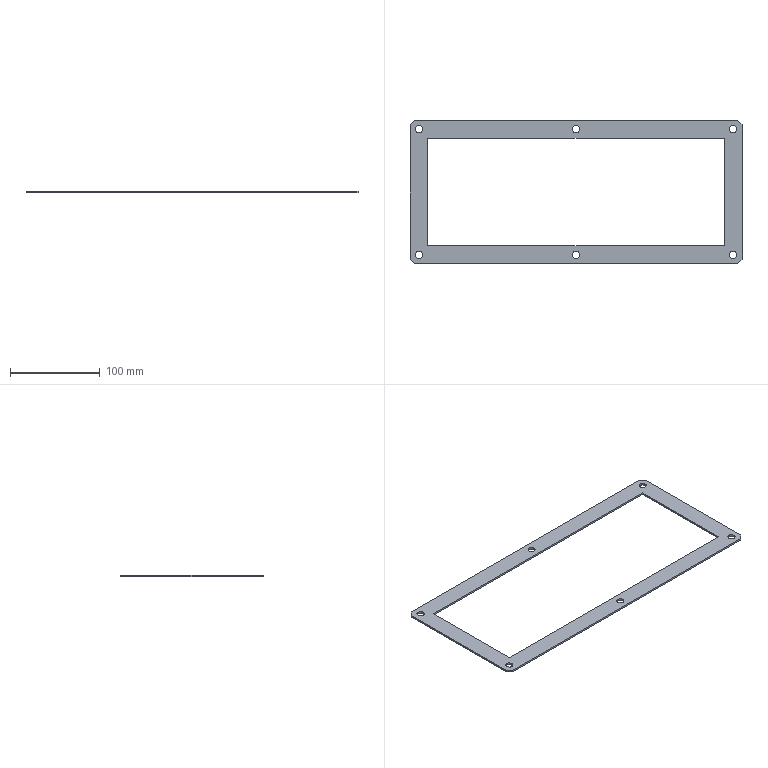Part | STEP file | SYL_0392D6J1SYL0380DJ10-1368501 | 1 solid | 26 faces | box 370 x 160 x 2 mm | volume 38497 mm3 | plane 14 | cylinder 12 | commonest cylinder face diameters 8 x12
STEP:
#1=CARTESIAN_POINT('',(-171.,70.,-2.));
#2=VERTEX_POINT('',#1);
#3=CARTESIAN_POINT('',(-179.,70.,-2.));
#4=VERTEX_POINT('',#3);
#5=CARTESIAN_POINT('',(-175.,70.,-2.));
#6=DIRECTION('',(0.,0.,1.));
#7=DIRECTION('',(1.,0.,0.));
#8=AXIS2_PLACEMENT_3D('',#5,#6,#7);
#9=CIRCLE('',#8,4.);
#10=EDGE_CURVE('',#2,#4,#9,.T.);
#11=ORIENTED_EDGE('',*,*,#10,.F.);
#12=CARTESIAN_POINT('',(-171.,70.,0.));
#13=VERTEX_POINT('',#12);
#14=CARTESIAN_POINT('',(-171.,70.,0.));
#15=DIRECTION('',(0.,0.,-1.));
#16=VECTOR('',#15,1000.);
#17=LINE('',#14,#16);
#18=EDGE_CURVE('',#13,#2,#17,.T.);
#19=ORIENTED_EDGE('',*,*,#18,.F.);
#20=CARTESIAN_POINT('',(-179.,70.,0.));
#21=VERTEX_POINT('',#20);
#22=CARTESIAN_POINT('',(-175.,70.,0.));
#23=DIRECTION('',(0.,0.,-1.));
#24=DIRECTION('',(-1.,0.,0.));
#25=AXIS2_PLACEMENT_3D('',#22,#23,#24);
#26=CIRCLE('',#25,4.);
#27=EDGE_CURVE('',#21,#13,#26,.T.);
#28=ORIENTED_EDGE('',*,*,#27,.F.);
#29=CARTESIAN_POINT('',(-179.,70.,0.));
#30=DIRECTION('',(0.,0.,-1.));
#31=VECTOR('',#30,1000.);
#32=LINE('',#29,#31);
#33=EDGE_CURVE('',#21,#4,#32,.T.);
#34=ORIENTED_EDGE('',*,*,#33,.T.);
#35=EDGE_LOOP('',(#11,#19,#28,#34));
#36=FACE_OUTER_BOUND('',#35,.T.);
#37=CARTESIAN_POINT('',(-175.,70.,-1.));
#38=DIRECTION('',(0.,0.,1.));
#39=DIRECTION('',(1.,0.,0.));
#40=AXIS2_PLACEMENT_3D('',#37,#38,#39);
#41=CYLINDRICAL_SURFACE('',#40,4.);
#42=ADVANCED_FACE('',(#36),#41,.F.);
#43=ORIENTED_EDGE('',*,*,#33,.F.);
#44=CARTESIAN_POINT('',(-175.,70.,0.));
#45=DIRECTION('',(0.,0.,-1.));
#46=DIRECTION('',(1.,0.,0.));
#47=AXIS2_PLACEMENT_3D('',#44,#45,#46);
#48=CIRCLE('',#47,4.);
#49=EDGE_CURVE('',#13,#21,#48,.T.);
#50=ORIENTED_EDGE('',*,*,#49,.F.);
#51=ORIENTED_EDGE('',*,*,#18,.T.);
#52=CARTESIAN_POINT('',(-175.,70.,-2.));
#53=DIRECTION('',(0.,0.,1.));
#54=DIRECTION('',(-1.,0.,0.));
#55=AXIS2_PLACEMENT_3D('',#52,#53,#54);
#56=CIRCLE('',#55,4.);
#57=EDGE_CURVE('',#4,#2,#56,.T.);
#58=ORIENTED_EDGE('',*,*,#57,.F.);
#59=EDGE_LOOP('',(#43,#50,#51,#58));
#60=FACE_OUTER_BOUND('',#59,.T.);
#61=CARTESIAN_POINT('',(-175.,70.,-1.));
#62=DIRECTION('',(0.,0.,1.));
#63=DIRECTION('',(1.,0.,0.));
#64=AXIS2_PLACEMENT_3D('',#61,#62,#63);
#65=CYLINDRICAL_SURFACE('',#64,4.);
#66=ADVANCED_FACE('',(#60),#65,.F.);
#67=CARTESIAN_POINT('',(165.,-60.,0.));
#68=VERTEX_POINT('',#67);
#69=CARTESIAN_POINT('',(-165.,-60.,0.));
#70=VERTEX_POINT('',#69);
#71=CARTESIAN_POINT('',(165.,-60.,0.));
#72=DIRECTION('',(-1.,0.,0.));
#73=VECTOR('',#72,1000.);
#74=LINE('',#71,#73);
#75=EDGE_CURVE('',#68,#70,#74,.T.);
#76=ORIENTED_EDGE('',*,*,#75,.F.);
#77=CARTESIAN_POINT('',(165.,-60.,-2.));
#78=VERTEX_POINT('',#77);
#79=CARTESIAN_POINT('',(165.,-60.,-2.));
#80=DIRECTION('',(0.,0.,1.));
#81=VECTOR('',#80,1000.);
#82=LINE('',#79,#81);
#83=EDGE_CURVE('',#78,#68,#82,.T.);
#84=ORIENTED_EDGE('',*,*,#83,.F.);
#85=CARTESIAN_POINT('',(-165.,-60.,-2.));
#86=VERTEX_POINT('',#85);
#87=CARTESIAN_POINT('',(-165.,-60.,-2.));
#88=DIRECTION('',(1.,0.,0.));
#89=VECTOR('',#88,1000.);
#90=LINE('',#87,#89);
#91=EDGE_CURVE('',#86,#78,#90,.T.);
#92=ORIENTED_EDGE('',*,*,#91,.F.);
#93=CARTESIAN_POINT('',(-165.,-60.,-2.));
#94=DIRECTION('',(0.,0.,1.));
#95=VECTOR('',#94,1000.);
#96=LINE('',#93,#95);
#97=EDGE_CURVE('',#86,#70,#96,.T.);
#98=ORIENTED_EDGE('',*,*,#97,.T.);
#99=EDGE_LOOP('',(#76,#84,#92,#98));
#100=FACE_OUTER_BOUND('',#99,.T.);
#101=CARTESIAN_POINT('',(0.,-60.,-1.));
#102=DIRECTION('',(0.,1.,0.));
#103=DIRECTION('',(1.,0.,0.));
#104=AXIS2_PLACEMENT_3D('',#101,#102,#103);
#105=PLANE('',#104);
#106=ADVANCED_FACE('',(#100),#105,.T.);
#107=CARTESIAN_POINT('',(165.,60.,0.));
#108=VERTEX_POINT('',#107);
#109=CARTESIAN_POINT('',(165.,60.,0.));
#110=DIRECTION('',(0.,-1.,0.));
#111=VECTOR('',#110,1000.);
#112=LINE('',#109,#111);
#113=EDGE_CURVE('',#108,#68,#112,.T.);
#114=ORIENTED_EDGE('',*,*,#113,.F.);
#115=CARTESIAN_POINT('',(165.,60.,-2.));
#116=VERTEX_POINT('',#115);
#117=CARTESIAN_POINT('',(165.,60.,-2.));
#118=DIRECTION('',(0.,0.,1.));
#119=VECTOR('',#118,1000.);
#120=LINE('',#117,#119);
#121=EDGE_CURVE('',#116,#108,#120,.T.);
#122=ORIENTED_EDGE('',*,*,#121,.F.);
#123=CARTESIAN_POINT('',(165.,-60.,-2.));
#124=DIRECTION('',(0.,1.,0.));
#125=VECTOR('',#124,1000.);
#126=LINE('',#123,#125);
#127=EDGE_CURVE('',#78,#116,#126,.T.);
#128=ORIENTED_EDGE('',*,*,#127,.F.);
#129=ORIENTED_EDGE('',*,*,#83,.T.);
#130=EDGE_LOOP('',(#114,#122,#128,#129));
#131=FACE_OUTER_BOUND('',#130,.T.);
#132=CARTESIAN_POINT('',(165.,0.,-1.));
#133=DIRECTION('',(-1.,0.,0.));
#134=DIRECTION('',(0.,0.,1.));
#135=AXIS2_PLACEMENT_3D('',#132,#133,#134);
#136=PLANE('',#135);
#137=ADVANCED_FACE('',(#131),#136,.T.);
#138=CARTESIAN_POINT('',(-165.,60.,0.));
#139=VERTEX_POINT('',#138);
#140=CARTESIAN_POINT('',(-165.,60.,0.));
#141=DIRECTION('',(1.,0.,0.));
#142=VECTOR('',#141,1000.);
#143=LINE('',#140,#142);
#144=EDGE_CURVE('',#139,#108,#143,.T.);
#145=ORIENTED_EDGE('',*,*,#144,.F.);
#146=CARTESIAN_POINT('',(-165.,60.,-2.));
#147=VERTEX_POINT('',#146);
#148=CARTESIAN_POINT('',(-165.,60.,0.));
#149=DIRECTION('',(0.,0.,-1.));
#150=VECTOR('',#149,1000.);
#151=LINE('',#148,#150);
#152=EDGE_CURVE('',#139,#147,#151,.T.);
#153=ORIENTED_EDGE('',*,*,#152,.T.);
#154=CARTESIAN_POINT('',(165.,60.,-2.));
#155=DIRECTION('',(-1.,0.,0.));
#156=VECTOR('',#155,1000.);
#157=LINE('',#154,#156);
#158=EDGE_CURVE('',#116,#147,#157,.T.);
#159=ORIENTED_EDGE('',*,*,#158,.F.);
#160=ORIENTED_EDGE('',*,*,#121,.T.);
#161=EDGE_LOOP('',(#145,#153,#159,#160));
#162=FACE_OUTER_BOUND('',#161,.T.);
#163=CARTESIAN_POINT('',(0.,60.,-1.));
#164=DIRECTION('',(0.,-1.,0.));
#165=DIRECTION('',(0.,0.,-1.));
#166=AXIS2_PLACEMENT_3D('',#163,#164,#165);
#167=PLANE('',#166);
#168=ADVANCED_FACE('',(#162),#167,.T.);
#169=CARTESIAN_POINT('',(-165.,-60.,0.));
#170=DIRECTION('',(0.,1.,0.));
#171=VECTOR('',#170,1000.);
#172=LINE('',#169,#171);
#173=EDGE_CURVE('',#70,#139,#172,.T.);
#174=ORIENTED_EDGE('',*,*,#173,.F.);
#175=ORIENTED_EDGE('',*,*,#97,.F.);
#176=CARTESIAN_POINT('',(-165.,60.,-2.));
#177=DIRECTION('',(0.,-1.,0.));
#178=VECTOR('',#177,1000.);
#179=LINE('',#176,#178);
#180=EDGE_CURVE('',#147,#86,#179,.T.);
#181=ORIENTED_EDGE('',*,*,#180,.F.);
#182=ORIENTED_EDGE('',*,*,#152,.F.);
#183=EDGE_LOOP('',(#174,#175,#181,#182));
#184=FACE_OUTER_BOUND('',#183,.T.);
#185=CARTESIAN_POINT('',(-165.,0.,-1.));
#186=DIRECTION('',(1.,0.,0.));
#187=DIRECTION('',(0.,1.,0.));
#188=AXIS2_PLACEMENT_3D('',#185,#186,#187);
#189=PLANE('',#188);
#190=ADVANCED_FACE('',(#184),#189,.T.);
#191=CARTESIAN_POINT('',(179.,-70.,-2.));
#192=VERTEX_POINT('',#191);
#193=CARTESIAN_POINT('',(171.,-70.,-2.));
#194=VERTEX_POINT('',#193);
#195=CARTESIAN_POINT('',(175.,-70.,-2.));
#196=DIRECTION('',(0.,0.,1.));
#197=DIRECTION('',(1.,0.,0.));
#198=AXIS2_PLACEMENT_3D('',#195,#196,#197);
#199=CIRCLE('',#198,4.);
#200=EDGE_CURVE('',#192,#194,#199,.T.);
#201=ORIENTED_EDGE('',*,*,#200,.F.);
#202=CARTESIAN_POINT('',(179.,-70.,0.));
#203=VERTEX_POINT('',#202);
#204=CARTESIAN_POINT('',(179.,-70.,0.));
#205=DIRECTION('',(0.,0.,-1.));
#206=VECTOR('',#205,1000.);
#207=LINE('',#204,#206);
#208=EDGE_CURVE('',#203,#192,#207,.T.);
#209=ORIENTED_EDGE('',*,*,#208,.F.);
#210=CARTESIAN_POINT('',(171.,-70.,0.));
#211=VERTEX_POINT('',#210);
#212=CARTESIAN_POINT('',(175.,-70.,0.));
#213=DIRECTION('',(0.,0.,-1.));
#214=DIRECTION('',(-1.,0.,0.));
#215=AXIS2_PLACEMENT_3D('',#212,#213,#214);
#216=CIRCLE('',#215,4.);
#217=EDGE_CURVE('',#211,#203,#216,.T.);
#218=ORIENTED_EDGE('',*,*,#217,.F.);
#219=CARTESIAN_POINT('',(171.,-70.,0.));
#220=DIRECTION('',(0.,0.,-1.));
#221=VECTOR('',#220,1000.);
#222=LINE('',#219,#221);
#223=EDGE_CURVE('',#211,#194,#222,.T.);
#224=ORIENTED_EDGE('',*,*,#223,.T.);
#225=EDGE_LOOP('',(#201,#209,#218,#224));
#226=FACE_OUTER_BOUND('',#225,.T.);
#227=CARTESIAN_POINT('',(175.,-70.,-1.));
#228=DIRECTION('',(0.,0.,1.));
#229=DIRECTION('',(1.,0.,0.));
#230=AXIS2_PLACEMENT_3D('',#227,#228,#229);
#231=CYLINDRICAL_SURFACE('',#230,4.);
#232=ADVANCED_FACE('',(#226),#231,.F.);
#233=CARTESIAN_POINT('',(4.,-70.,-2.));
#234=VERTEX_POINT('',#233);
#235=CARTESIAN_POINT('',(-4.,-70.,-2.));
#236=VERTEX_POINT('',#235);
#237=CARTESIAN_POINT('',(0.,-70.,-2.));
#238=DIRECTION('',(0.,0.,1.));
#239=DIRECTION('',(1.,0.,0.));
#240=AXIS2_PLACEMENT_3D('',#237,#238,#239);
#241=CIRCLE('',#240,4.);
#242=EDGE_CURVE('',#234,#236,#241,.T.);
#243=ORIENTED_EDGE('',*,*,#242,.F.);
#244=CARTESIAN_POINT('',(4.,-70.,0.));
#245=VERTEX_POINT('',#244);
#246=CARTESIAN_POINT('',(4.,-70.,0.));
#247=DIRECTION('',(0.,0.,-1.));
#248=VECTOR('',#247,1000.);
#249=LINE('',#246,#248);
#250=EDGE_CURVE('',#245,#234,#249,.T.);
#251=ORIENTED_EDGE('',*,*,#250,.F.);
#252=CARTESIAN_POINT('',(-4.,-70.,0.));
#253=VERTEX_POINT('',#252);
#254=CARTESIAN_POINT('',(0.,-70.,0.));
#255=DIRECTION('',(0.,0.,-1.));
#256=DIRECTION('',(-1.,0.,0.));
#257=AXIS2_PLACEMENT_3D('',#254,#255,#256);
#258=CIRCLE('',#257,4.);
#259=EDGE_CURVE('',#253,#245,#258,.T.);
#260=ORIENTED_EDGE('',*,*,#259,.F.);
#261=CARTESIAN_POINT('',(-4.,-70.,0.));
#262=DIRECTION('',(0.,0.,-1.));
#263=VECTOR('',#262,1000.);
#264=LINE('',#261,#263);
#265=EDGE_CURVE('',#253,#236,#264,.T.);
#266=ORIENTED_EDGE('',*,*,#265,.T.);
#267=EDGE_LOOP('',(#243,#251,#260,#266));
#268=FACE_OUTER_BOUND('',#267,.T.);
#269=CARTESIAN_POINT('',(0.,-70.,-1.));
#270=DIRECTION('',(0.,0.,1.));
#271=DIRECTION('',(1.,0.,0.));
#272=AXIS2_PLACEMENT_3D('',#269,#270,#271);
#273=CYLINDRICAL_SURFACE('',#272,4.);
#274=ADVANCED_FACE('',(#268),#273,.F.);
#275=ORIENTED_EDGE('',*,*,#265,.F.);
#276=CARTESIAN_POINT('',(0.,-70.,0.));
#277=DIRECTION('',(0.,0.,-1.));
#278=DIRECTION('',(1.,0.,0.));
#279=AXIS2_PLACEMENT_3D('',#276,#277,#278);
#280=CIRCLE('',#279,4.);
#281=EDGE_CURVE('',#245,#253,#280,.T.);
#282=ORIENTED_EDGE('',*,*,#281,.F.);
#283=ORIENTED_EDGE('',*,*,#250,.T.);
#284=CARTESIAN_POINT('',(0.,-70.,-2.));
#285=DIRECTION('',(0.,0.,1.));
#286=DIRECTION('',(-1.,0.,0.));
#287=AXIS2_PLACEMENT_3D('',#284,#285,#286);
#288=CIRCLE('',#287,4.);
#289=EDGE_CURVE('',#236,#234,#288,.T.);
#290=ORIENTED_EDGE('',*,*,#289,.F.);
#291=EDGE_LOOP('',(#275,#282,#283,#290));
#292=FACE_OUTER_BOUND('',#291,.T.);
#293=CARTESIAN_POINT('',(0.,-70.,-1.));
#294=DIRECTION('',(0.,0.,1.));
#295=DIRECTION('',(1.,0.,0.));
#296=AXIS2_PLACEMENT_3D('',#293,#294,#295);
#297=CYLINDRICAL_SURFACE('',#296,4.);
#298=ADVANCED_FACE('',(#292),#297,.F.);
#299=CARTESIAN_POINT('',(-171.,-70.,-2.));
#300=VERTEX_POINT('',#299);
#301=CARTESIAN_POINT('',(-179.,-70.,-2.));
#302=VERTEX_POINT('',#301);
#303=CARTESIAN_POINT('',(-175.,-70.,-2.));
#304=DIRECTION('',(0.,0.,1.));
#305=DIRECTION('',(1.,0.,0.));
#306=AXIS2_PLACEMENT_3D('',#303,#304,#305);
#307=CIRCLE('',#306,4.);
#308=EDGE_CURVE('',#300,#302,#307,.T.);
#309=ORIENTED_EDGE('',*,*,#308,.F.);
#310=CARTESIAN_POINT('',(-171.,-70.,0.));
#311=VERTEX_POINT('',#310);
#312=CARTESIAN_POINT('',(-171.,-70.,0.));
#313=DIRECTION('',(0.,0.,-1.));
#314=VECTOR('',#313,1000.);
#315=LINE('',#312,#314);
#316=EDGE_CURVE('',#311,#300,#315,.T.);
#317=ORIENTED_EDGE('',*,*,#316,.F.);
#318=CARTESIAN_POINT('',(-179.,-70.,0.));
#319=VERTEX_POINT('',#318);
#320=CARTESIAN_POINT('',(-175.,-70.,0.));
#321=DIRECTION('',(0.,0.,-1.));
#322=DIRECTION('',(-1.,0.,0.));
#323=AXIS2_PLACEMENT_3D('',#320,#321,#322);
#324=CIRCLE('',#323,4.);
#325=EDGE_CURVE('',#319,#311,#324,.T.);
#326=ORIENTED_EDGE('',*,*,#325,.F.);
#327=CARTESIAN_POINT('',(-179.,-70.,0.));
#328=DIRECTION('',(0.,0.,-1.));
#329=VECTOR('',#328,1000.);
#330=LINE('',#327,#329);
#331=EDGE_CURVE('',#319,#302,#330,.T.);
#332=ORIENTED_EDGE('',*,*,#331,.T.);
#333=EDGE_LOOP('',(#309,#317,#326,#332));
#334=FACE_OUTER_BOUND('',#333,.T.);
#335=CARTESIAN_POINT('',(-175.,-70.,-1.));
#336=DIRECTION('',(0.,0.,1.));
#337=DIRECTION('',(1.,0.,0.));
#338=AXIS2_PLACEMENT_3D('',#335,#336,#337);
#339=CYLINDRICAL_SURFACE('',#338,4.);
#340=ADVANCED_FACE('',(#334),#339,.F.);
#341=ORIENTED_EDGE('',*,*,#331,.F.);
#342=CARTESIAN_POINT('',(-175.,-70.,0.));
#343=DIRECTION('',(0.,0.,-1.));
#344=DIRECTION('',(1.,0.,0.));
#345=AXIS2_PLACEMENT_3D('',#342,#343,#344);
#346=CIRCLE('',#345,4.);
#347=EDGE_CURVE('',#311,#319,#346,.T.);
#348=ORIENTED_EDGE('',*,*,#347,.F.);
#349=ORIENTED_EDGE('',*,*,#316,.T.);
#350=CARTESIAN_POINT('',(-175.,-70.,-2.));
#351=DIRECTION('',(0.,0.,1.));
#352=DIRECTION('',(-1.,0.,0.));
#353=AXIS2_PLACEMENT_3D('',#350,#351,#352);
#354=CIRCLE('',#353,4.);
#355=EDGE_CURVE('',#302,#300,#354,.T.);
#356=ORIENTED_EDGE('',*,*,#355,.F.);
#357=EDGE_LOOP('',(#341,#348,#349,#356));
#358=FACE_OUTER_BOUND('',#357,.T.);
#359=CARTESIAN_POINT('',(-175.,-70.,-1.));
#360=DIRECTION('',(0.,0.,1.));
#361=DIRECTION('',(1.,0.,0.));
#362=AXIS2_PLACEMENT_3D('',#359,#360,#361);
#363=CYLINDRICAL_SURFACE('',#362,4.);
#364=ADVANCED_FACE('',(#358),#363,.F.);
#365=CARTESIAN_POINT('',(179.,70.,-2.));
#366=VERTEX_POINT('',#365);
#367=CARTESIAN_POINT('',(171.,70.,-2.));
#368=VERTEX_POINT('',#367);
#369=CARTESIAN_POINT('',(175.,70.,-2.));
#370=DIRECTION('',(0.,0.,1.));
#371=DIRECTION('',(1.,0.,0.));
#372=AXIS2_PLACEMENT_3D('',#369,#370,#371);
#373=CIRCLE('',#372,4.);
#374=EDGE_CURVE('',#366,#368,#373,.T.);
#375=ORIENTED_EDGE('',*,*,#374,.F.);
#376=CARTESIAN_POINT('',(179.,70.,0.));
#377=VERTEX_POINT('',#376);
#378=CARTESIAN_POINT('',(179.,70.,0.));
#379=DIRECTION('',(0.,0.,-1.));
#380=VECTOR('',#379,1000.);
#381=LINE('',#378,#380);
#382=EDGE_CURVE('',#377,#366,#381,.T.);
#383=ORIENTED_EDGE('',*,*,#382,.F.);
#384=CARTESIAN_POINT('',(171.,70.,0.));
#385=VERTEX_POINT('',#384);
#386=CARTESIAN_POINT('',(175.,70.,0.));
#387=DIRECTION('',(0.,0.,-1.));
#388=DIRECTION('',(-1.,0.,0.));
#389=AXIS2_PLACEMENT_3D('',#386,#387,#388);
#390=CIRCLE('',#389,4.);
#391=EDGE_CURVE('',#385,#377,#390,.T.);
#392=ORIENTED_EDGE('',*,*,#391,.F.);
#393=CARTESIAN_POINT('',(171.,70.,0.));
#394=DIRECTION('',(0.,0.,-1.));
#395=VECTOR('',#394,1000.);
#396=LINE('',#393,#395);
#397=EDGE_CURVE('',#385,#368,#396,.T.);
#398=ORIENTED_EDGE('',*,*,#397,.T.);
#399=EDGE_LOOP('',(#375,#383,#392,#398));
#400=FACE_OUTER_BOUND('',#399,.T.);
#401=CARTESIAN_POINT('',(175.,70.,-1.));
#402=DIRECTION('',(0.,0.,1.));
#403=DIRECTION('',(1.,0.,0.));
#404=AXIS2_PLACEMENT_3D('',#401,#402,#403);
#405=CYLINDRICAL_SURFACE('',#404,4.);
#406=ADVANCED_FACE('',(#400),#405,.F.);
#407=ORIENTED_EDGE('',*,*,#397,.F.);
#408=CARTESIAN_POINT('',(175.,70.,0.));
#409=DIRECTION('',(0.,0.,-1.));
#410=DIRECTION('',(1.,0.,0.));
#411=AXIS2_PLACEMENT_3D('',#408,#409,#410);
#412=CIRCLE('',#411,4.);
#413=EDGE_CURVE('',#377,#385,#412,.T.);
#414=ORIENTED_EDGE('',*,*,#413,.F.);
#415=ORIENTED_EDGE('',*,*,#382,.T.);
#416=CARTESIAN_POINT('',(175.,70.,-2.));
#417=DIRECTION('',(0.,0.,1.));
#418=DIRECTION('',(-1.,0.,0.));
#419=AXIS2_PLACEMENT_3D('',#416,#417,#418);
#420=CIRCLE('',#419,4.);
#421=EDGE_CURVE('',#368,#366,#420,.T.);
#422=ORIENTED_EDGE('',*,*,#421,.F.);
#423=EDGE_LOOP('',(#407,#414,#415,#422));
#424=FACE_OUTER_BOUND('',#423,.T.);
#425=CARTESIAN_POINT('',(175.,70.,-1.));
#426=DIRECTION('',(0.,0.,1.));
#427=DIRECTION('',(1.,0.,0.));
#428=AXIS2_PLACEMENT_3D('',#425,#426,#427);
#429=CYLINDRICAL_SURFACE('',#428,4.);
#430=ADVANCED_FACE('',(#424),#429,.F.);
#431=CARTESIAN_POINT('',(4.,70.,-2.));
#432=VERTEX_POINT('',#431);
#433=CARTESIAN_POINT('',(-4.,70.,-2.));
#434=VERTEX_POINT('',#433);
#435=CARTESIAN_POINT('',(0.,70.,-2.));
#436=DIRECTION('',(0.,0.,1.));
#437=DIRECTION('',(1.,0.,0.));
#438=AXIS2_PLACEMENT_3D('',#435,#436,#437);
#439=CIRCLE('',#438,4.);
#440=EDGE_CURVE('',#432,#434,#439,.T.);
#441=ORIENTED_EDGE('',*,*,#440,.F.);
#442=CARTESIAN_POINT('',(4.,70.,0.));
#443=VERTEX_POINT('',#442);
#444=CARTESIAN_POINT('',(4.,70.,0.));
#445=DIRECTION('',(0.,0.,-1.));
#446=VECTOR('',#445,1000.);
#447=LINE('',#444,#446);
#448=EDGE_CURVE('',#443,#432,#447,.T.);
#449=ORIENTED_EDGE('',*,*,#448,.F.);
#450=CARTESIAN_POINT('',(-4.,70.,0.));
#451=VERTEX_POINT('',#450);
#452=CARTESIAN_POINT('',(0.,70.,0.));
#453=DIRECTION('',(0.,0.,-1.));
#454=DIRECTION('',(-1.,0.,0.));
#455=AXIS2_PLACEMENT_3D('',#452,#453,#454);
#456=CIRCLE('',#455,4.);
#457=EDGE_CURVE('',#451,#443,#456,.T.);
#458=ORIENTED_EDGE('',*,*,#457,.F.);
#459=CARTESIAN_POINT('',(-4.,70.,0.));
#460=DIRECTION('',(0.,0.,-1.));
#461=VECTOR('',#460,1000.);
#462=LINE('',#459,#461);
#463=EDGE_CURVE('',#451,#434,#462,.T.);
#464=ORIENTED_EDGE('',*,*,#463,.T.);
#465=EDGE_LOOP('',(#441,#449,#458,#464));
#466=FACE_OUTER_BOUND('',#465,.T.);
#467=CARTESIAN_POINT('',(0.,70.,-1.));
#468=DIRECTION('',(0.,0.,1.));
#469=DIRECTION('',(1.,0.,0.));
#470=AXIS2_PLACEMENT_3D('',#467,#468,#469);
#471=CYLINDRICAL_SURFACE('',#470,4.);
#472=ADVANCED_FACE('',(#466),#471,.F.);
#473=ORIENTED_EDGE('',*,*,#463,.F.);
#474=CARTESIAN_POINT('',(0.,70.,0.));
#475=DIRECTION('',(0.,0.,-1.));
#476=DIRECTION('',(1.,0.,0.));
#477=AXIS2_PLACEMENT_3D('',#474,#475,#476);
#478=CIRCLE('',#477,4.);
#479=EDGE_CURVE('',#443,#451,#478,.T.);
#480=ORIENTED_EDGE('',*,*,#479,.F.);
#481=ORIENTED_EDGE('',*,*,#448,.T.);
#482=CARTESIAN_POINT('',(0.,70.,-2.));
#483=DIRECTION('',(0.,0.,1.));
#484=DIRECTION('',(-1.,0.,0.));
#485=AXIS2_PLACEMENT_3D('',#482,#483,#484);
#486=CIRCLE('',#485,4.);
#487=EDGE_CURVE('',#434,#432,#486,.T.);
#488=ORIENTED_EDGE('',*,*,#487,.F.);
#489=EDGE_LOOP('',(#473,#480,#481,#488));
#490=FACE_OUTER_BOUND('',#489,.T.);
#491=CARTESIAN_POINT('',(0.,70.,-1.));
#492=DIRECTION('',(0.,0.,1.));
#493=DIRECTION('',(1.,0.,0.));
#494=AXIS2_PLACEMENT_3D('',#491,#492,#493);
#495=CYLINDRICAL_SURFACE('',#494,4.);
#496=ADVANCED_FACE('',(#490),#495,.F.);
#497=CARTESIAN_POINT('',(185.,75.,0.));
#498=VERTEX_POINT('',#497);
#499=CARTESIAN_POINT('',(180.,80.,0.));
#500=VERTEX_POINT('',#499);
#501=CARTESIAN_POINT('',(185.,75.,0.));
#502=DIRECTION('',(-0.7071,0.7071,0.));
#503=VECTOR('',#502,1000.);
#504=LINE('',#501,#503);
#505=EDGE_CURVE('',#498,#500,#504,.T.);
#506=ORIENTED_EDGE('',*,*,#505,.F.);
#507=CARTESIAN_POINT('',(185.,75.,-2.));
#508=VERTEX_POINT('',#507);
#509=CARTESIAN_POINT('',(185.,75.,0.));
#510=DIRECTION('',(0.,0.,-1.));
#511=VECTOR('',#510,1000.);
#512=LINE('',#509,#511);
#513=EDGE_CURVE('',#498,#508,#512,.T.);
#514=ORIENTED_EDGE('',*,*,#513,.T.);
#515=CARTESIAN_POINT('',(180.,80.,-2.));
#516=VERTEX_POINT('',#515);
#517=CARTESIAN_POINT('',(180.,80.,-2.));
#518=DIRECTION('',(0.7071,-0.7071,0.));
#519=VECTOR('',#518,1000.);
#520=LINE('',#517,#519);
#521=EDGE_CURVE('',#516,#508,#520,.T.);
#522=ORIENTED_EDGE('',*,*,#521,.F.);
#523=CARTESIAN_POINT('',(180.,80.,-2.));
#524=DIRECTION('',(0.,0.,1.));
#525=VECTOR('',#524,1000.);
#526=LINE('',#523,#525);
#527=EDGE_CURVE('',#516,#500,#526,.T.);
#528=ORIENTED_EDGE('',*,*,#527,.T.);
#529=EDGE_LOOP('',(#506,#514,#522,#528));
#530=FACE_OUTER_BOUND('',#529,.T.);
#531=CARTESIAN_POINT('',(182.5,77.5,-1.));
#532=DIRECTION('',(0.7071,0.7071,0.));
#533=DIRECTION('',(0.,0.,-1.));
#534=AXIS2_PLACEMENT_3D('',#531,#532,#533);
#535=PLANE('',#534);
#536=ADVANCED_FACE('',(#530),#535,.T.);
#537=ORIENTED_EDGE('',*,*,#527,.F.);
#538=CARTESIAN_POINT('',(-180.,80.,-2.));
#539=VERTEX_POINT('',#538);
#540=CARTESIAN_POINT('',(-180.,80.,-2.));
#541=DIRECTION('',(1.,0.,0.));
#542=VECTOR('',#541,1000.);
#543=LINE('',#540,#542);
#544=EDGE_CURVE('',#539,#516,#543,.T.);
#545=ORIENTED_EDGE('',*,*,#544,.F.);
#546=CARTESIAN_POINT('',(-180.,80.,0.));
#547=VERTEX_POINT('',#546);
#548=CARTESIAN_POINT('',(-180.,80.,-2.));
#549=DIRECTION('',(0.,0.,1.));
#550=VECTOR('',#549,1000.);
#551=LINE('',#548,#550);
#552=EDGE_CURVE('',#539,#547,#551,.T.);
#553=ORIENTED_EDGE('',*,*,#552,.T.);
#554=CARTESIAN_POINT('',(180.,80.,0.));
#555=DIRECTION('',(-1.,0.,0.));
#556=VECTOR('',#555,1000.);
#557=LINE('',#554,#556);
#558=EDGE_CURVE('',#500,#547,#557,.T.);
#559=ORIENTED_EDGE('',*,*,#558,.F.);
#560=EDGE_LOOP('',(#537,#545,#553,#559));
#561=FACE_OUTER_BOUND('',#560,.T.);
#562=CARTESIAN_POINT('',(0.,80.,-1.));
#563=DIRECTION('',(0.,1.,0.));
#564=DIRECTION('',(1.,0.,0.));
#565=AXIS2_PLACEMENT_3D('',#562,#563,#564);
#566=PLANE('',#565);
#567=ADVANCED_FACE('',(#561),#566,.T.);
#568=CARTESIAN_POINT('',(-185.,75.,0.));
#569=VERTEX_POINT('',#568);
#570=CARTESIAN_POINT('',(-180.,80.,0.));
#571=DIRECTION('',(-0.7071,-0.7071,0.));
#572=VECTOR('',#571,1000.);
#573=LINE('',#570,#572);
#574=EDGE_CURVE('',#547,#569,#573,.T.);
#575=ORIENTED_EDGE('',*,*,#574,.F.);
#576=ORIENTED_EDGE('',*,*,#552,.F.);
#577=CARTESIAN_POINT('',(-185.,75.,-2.));
#578=VERTEX_POINT('',#577);
#579=CARTESIAN_POINT('',(-185.,75.,-2.));
#580=DIRECTION('',(0.7071,0.7071,0.));
#581=VECTOR('',#580,1000.);
#582=LINE('',#579,#581);
#583=EDGE_CURVE('',#578,#539,#582,.T.);
#584=ORIENTED_EDGE('',*,*,#583,.F.);
#585=CARTESIAN_POINT('',(-185.,75.,-2.));
#586=DIRECTION('',(0.,0.,1.));
#587=VECTOR('',#586,1000.);
#588=LINE('',#585,#587);
#589=EDGE_CURVE('',#578,#569,#588,.T.);
#590=ORIENTED_EDGE('',*,*,#589,.T.);
#591=EDGE_LOOP('',(#575,#576,#584,#590));
#592=FACE_OUTER_BOUND('',#591,.T.);
#593=CARTESIAN_POINT('',(-182.5,77.5,-1.));
#594=DIRECTION('',(-0.7071,0.7071,0.));
#595=DIRECTION('',(0.,0.,1.));
#596=AXIS2_PLACEMENT_3D('',#593,#594,#595);
#597=PLANE('',#596);
#598=ADVANCED_FACE('',(#592),#597,.T.);
#599=ORIENTED_EDGE('',*,*,#589,.F.);
#600=CARTESIAN_POINT('',(-185.,-75.,-2.));
#601=VERTEX_POINT('',#600);
#602=CARTESIAN_POINT('',(-185.,-75.,-2.));
#603=DIRECTION('',(0.,1.,0.));
#604=VECTOR('',#603,1000.);
#605=LINE('',#602,#604);
#606=EDGE_CURVE('',#601,#578,#605,.T.);
#607=ORIENTED_EDGE('',*,*,#606,.F.);
#608=CARTESIAN_POINT('',(-185.,-75.,0.));
#609=VERTEX_POINT('',#608);
#610=CARTESIAN_POINT('',(-185.,-75.,-2.));
#611=DIRECTION('',(0.,0.,1.));
#612=VECTOR('',#611,1000.);
#613=LINE('',#610,#612);
#614=EDGE_CURVE('',#601,#609,#613,.T.);
#615=ORIENTED_EDGE('',*,*,#614,.T.);
#616=CARTESIAN_POINT('',(-185.,75.,0.));
#617=DIRECTION('',(0.,-1.,0.));
#618=VECTOR('',#617,1000.);
#619=LINE('',#616,#618);
#620=EDGE_CURVE('',#569,#609,#619,.T.);
#621=ORIENTED_EDGE('',*,*,#620,.F.);
#622=EDGE_LOOP('',(#599,#607,#615,#621));
#623=FACE_OUTER_BOUND('',#622,.T.);
#624=CARTESIAN_POINT('',(-185.,0.,-1.));
#625=DIRECTION('',(-1.,0.,0.));
#626=DIRECTION('',(0.,0.,1.));
#627=AXIS2_PLACEMENT_3D('',#624,#625,#626);
#628=PLANE('',#627);
#629=ADVANCED_FACE('',(#623),#628,.T.);
#630=CARTESIAN_POINT('',(-180.,-80.,0.));
#631=VERTEX_POINT('',#630);
#632=CARTESIAN_POINT('',(-185.,-75.,0.));
#633=DIRECTION('',(0.7071,-0.7071,0.));
#634=VECTOR('',#633,1000.);
#635=LINE('',#632,#634);
#636=EDGE_CURVE('',#609,#631,#635,.T.);
#637=ORIENTED_EDGE('',*,*,#636,.F.);
#638=ORIENTED_EDGE('',*,*,#614,.F.);
#639=CARTESIAN_POINT('',(-180.,-80.,-2.));
#640=VERTEX_POINT('',#639);
#641=CARTESIAN_POINT('',(-180.,-80.,-2.));
#642=DIRECTION('',(-0.7071,0.7071,0.));
#643=VECTOR('',#642,1000.);
#644=LINE('',#641,#643);
#645=EDGE_CURVE('',#640,#601,#644,.T.);
#646=ORIENTED_EDGE('',*,*,#645,.F.);
#647=CARTESIAN_POINT('',(-180.,-80.,-2.));
#648=DIRECTION('',(0.,0.,1.));
#649=VECTOR('',#648,1000.);
#650=LINE('',#647,#649);
#651=EDGE_CURVE('',#640,#631,#650,.T.);
#652=ORIENTED_EDGE('',*,*,#651,.T.);
#653=EDGE_LOOP('',(#637,#638,#646,#652));
#654=FACE_OUTER_BOUND('',#653,.T.);
#655=CARTESIAN_POINT('',(-182.5,-77.5,-1.));
#656=DIRECTION('',(-0.7071,-0.7071,0.));
#657=DIRECTION('',(-0.7071,0.7071,0.));
#658=AXIS2_PLACEMENT_3D('',#655,#656,#657);
#659=PLANE('',#658);
#660=ADVANCED_FACE('',(#654),#659,.T.);
#661=ORIENTED_EDGE('',*,*,#651,.F.);
#662=CARTESIAN_POINT('',(180.,-80.,-2.));
#663=VERTEX_POINT('',#662);
#664=CARTESIAN_POINT('',(180.,-80.,-2.));
#665=DIRECTION('',(-1.,0.,0.));
#666=VECTOR('',#665,1000.);
#667=LINE('',#664,#666);
#668=EDGE_CURVE('',#663,#640,#667,.T.);
#669=ORIENTED_EDGE('',*,*,#668,.F.);
#670=CARTESIAN_POINT('',(180.,-80.,0.));
#671=VERTEX_POINT('',#670);
#672=CARTESIAN_POINT('',(180.,-80.,-2.));
#673=DIRECTION('',(0.,0.,1.));
#674=VECTOR('',#673,1000.);
#675=LINE('',#672,#674);
#676=EDGE_CURVE('',#663,#671,#675,.T.);
#677=ORIENTED_EDGE('',*,*,#676,.T.);
#678=CARTESIAN_POINT('',(-180.,-80.,0.));
#679=DIRECTION('',(1.,0.,0.));
#680=VECTOR('',#679,1000.);
#681=LINE('',#678,#680);
#682=EDGE_CURVE('',#631,#671,#681,.T.);
#683=ORIENTED_EDGE('',*,*,#682,.F.);
#684=EDGE_LOOP('',(#661,#669,#677,#683));
#685=FACE_OUTER_BOUND('',#684,.T.);
#686=CARTESIAN_POINT('',(0.,-80.,-1.));
#687=DIRECTION('',(0.,-1.,0.));
#688=DIRECTION('',(0.,0.,-1.));
#689=AXIS2_PLACEMENT_3D('',#686,#687,#688);
#690=PLANE('',#689);
#691=ADVANCED_FACE('',(#685),#690,.T.);
#692=ORIENTED_EDGE('',*,*,#27,.T.);
#693=ORIENTED_EDGE('',*,*,#49,.T.);
#694=EDGE_LOOP('',(#692,#693));
#695=FACE_BOUND('',#694,.T.);
#696=ORIENTED_EDGE('',*,*,#144,.T.);
#697=ORIENTED_EDGE('',*,*,#113,.T.);
#698=ORIENTED_EDGE('',*,*,#75,.T.);
#699=ORIENTED_EDGE('',*,*,#173,.T.);
#700=EDGE_LOOP('',(#696,#697,#698,#699));
#701=FACE_BOUND('',#700,.T.);
#702=ORIENTED_EDGE('',*,*,#217,.T.);
#703=CARTESIAN_POINT('',(175.,-70.,0.));
#704=DIRECTION('',(0.,0.,-1.));
#705=DIRECTION('',(1.,0.,0.));
#706=AXIS2_PLACEMENT_3D('',#703,#704,#705);
#707=CIRCLE('',#706,4.);
#708=EDGE_CURVE('',#203,#211,#707,.T.);
#709=ORIENTED_EDGE('',*,*,#708,.T.);
#710=EDGE_LOOP('',(#702,#709));
#711=FACE_BOUND('',#710,.T.);
#712=ORIENTED_EDGE('',*,*,#259,.T.);
#713=ORIENTED_EDGE('',*,*,#281,.T.);
#714=EDGE_LOOP('',(#712,#713));
#715=FACE_BOUND('',#714,.T.);
#716=ORIENTED_EDGE('',*,*,#325,.T.);
#717=ORIENTED_EDGE('',*,*,#347,.T.);
#718=EDGE_LOOP('',(#716,#717));
#719=FACE_BOUND('',#718,.T.);
#720=ORIENTED_EDGE('',*,*,#391,.T.);
#721=ORIENTED_EDGE('',*,*,#413,.T.);
#722=EDGE_LOOP('',(#720,#721));
#723=FACE_BOUND('',#722,.T.);
#724=ORIENTED_EDGE('',*,*,#457,.T.);
#725=ORIENTED_EDGE('',*,*,#479,.T.);
#726=EDGE_LOOP('',(#724,#725));
#727=FACE_BOUND('',#726,.T.);
#728=ORIENTED_EDGE('',*,*,#505,.T.);
#729=ORIENTED_EDGE('',*,*,#558,.T.);
#730=ORIENTED_EDGE('',*,*,#574,.T.);
#731=ORIENTED_EDGE('',*,*,#620,.T.);
#732=ORIENTED_EDGE('',*,*,#636,.T.);
#733=ORIENTED_EDGE('',*,*,#682,.T.);
#734=CARTESIAN_POINT('',(185.,-75.,0.));
#735=VERTEX_POINT('',#734);
#736=CARTESIAN_POINT('',(180.,-80.,0.));
#737=DIRECTION('',(0.7071,0.7071,0.));
#738=VECTOR('',#737,1000.);
#739=LINE('',#736,#738);
#740=EDGE_CURVE('',#671,#735,#739,.T.);
#741=ORIENTED_EDGE('',*,*,#740,.T.);
#742=CARTESIAN_POINT('',(185.,-75.,0.));
#743=DIRECTION('',(0.,1.,0.));
#744=VECTOR('',#743,1000.);
#745=LINE('',#742,#744);
#746=EDGE_CURVE('',#735,#498,#745,.T.);
#747=ORIENTED_EDGE('',*,*,#746,.T.);
#748=EDGE_LOOP('',(#728,#729,#730,#731,#732,#733,#741,#747));
#749=FACE_OUTER_BOUND('',#748,.T.);
#750=CARTESIAN_POINT('',(0.,0.,0.));
#751=DIRECTION('',(0.,0.,1.));
#752=DIRECTION('',(1.,0.,0.));
#753=AXIS2_PLACEMENT_3D('',#750,#751,#752);
#754=PLANE('',#753);
#755=ADVANCED_FACE('',(#695,#701,#711,#715,#719,#723,#727,#749),#754,.T.);
#756=ORIENTED_EDGE('',*,*,#513,.F.);
#757=ORIENTED_EDGE('',*,*,#746,.F.);
#758=CARTESIAN_POINT('',(185.,-75.,-2.));
#759=VERTEX_POINT('',#758);
#760=CARTESIAN_POINT('',(185.,-75.,-2.));
#761=DIRECTION('',(0.,0.,1.));
#762=VECTOR('',#761,1000.);
#763=LINE('',#760,#762);
#764=EDGE_CURVE('',#759,#735,#763,.T.);
#765=ORIENTED_EDGE('',*,*,#764,.F.);
#766=CARTESIAN_POINT('',(185.,75.,-2.));
#767=DIRECTION('',(0.,-1.,0.));
#768=VECTOR('',#767,1000.);
#769=LINE('',#766,#768);
#770=EDGE_CURVE('',#508,#759,#769,.T.);
#771=ORIENTED_EDGE('',*,*,#770,.F.);
#772=EDGE_LOOP('',(#756,#757,#765,#771));
#773=FACE_OUTER_BOUND('',#772,.T.);
#774=CARTESIAN_POINT('',(185.,0.,-1.));
#775=DIRECTION('',(1.,0.,0.));
#776=DIRECTION('',(0.,1.,0.));
#777=AXIS2_PLACEMENT_3D('',#774,#775,#776);
#778=PLANE('',#777);
#779=ADVANCED_FACE('',(#773),#778,.T.);
#780=ORIENTED_EDGE('',*,*,#740,.F.);
#781=ORIENTED_EDGE('',*,*,#676,.F.);
#782=CARTESIAN_POINT('',(185.,-75.,-2.));
#783=DIRECTION('',(-0.7071,-0.7071,0.));
#784=VECTOR('',#783,1000.);
#785=LINE('',#782,#784);
#786=EDGE_CURVE('',#759,#663,#785,.T.);
#787=ORIENTED_EDGE('',*,*,#786,.F.);
#788=ORIENTED_EDGE('',*,*,#764,.T.);
#789=EDGE_LOOP('',(#780,#781,#787,#788));
#790=FACE_OUTER_BOUND('',#789,.T.);
#791=CARTESIAN_POINT('',(182.5,-77.5,-1.));
#792=DIRECTION('',(0.7071,-0.7071,0.));
#793=DIRECTION('',(0.,0.,-1.));
#794=AXIS2_PLACEMENT_3D('',#791,#792,#793);
#795=PLANE('',#794);
#796=ADVANCED_FACE('',(#790),#795,.T.);
#797=ORIENTED_EDGE('',*,*,#10,.T.);
#798=ORIENTED_EDGE('',*,*,#57,.T.);
#799=EDGE_LOOP('',(#797,#798));
#800=FACE_BOUND('',#799,.T.);
#801=ORIENTED_EDGE('',*,*,#127,.T.);
#802=ORIENTED_EDGE('',*,*,#158,.T.);
#803=ORIENTED_EDGE('',*,*,#180,.T.);
#804=ORIENTED_EDGE('',*,*,#91,.T.);
#805=EDGE_LOOP('',(#801,#802,#803,#804));
#806=FACE_BOUND('',#805,.T.);
#807=ORIENTED_EDGE('',*,*,#200,.T.);
#808=CARTESIAN_POINT('',(175.,-70.,-2.));
#809=DIRECTION('',(0.,0.,1.));
#810=DIRECTION('',(-1.,0.,0.));
#811=AXIS2_PLACEMENT_3D('',#808,#809,#810);
#812=CIRCLE('',#811,4.);
#813=EDGE_CURVE('',#194,#192,#812,.T.);
#814=ORIENTED_EDGE('',*,*,#813,.T.);
#815=EDGE_LOOP('',(#807,#814));
#816=FACE_BOUND('',#815,.T.);
#817=ORIENTED_EDGE('',*,*,#242,.T.);
#818=ORIENTED_EDGE('',*,*,#289,.T.);
#819=EDGE_LOOP('',(#817,#818));
#820=FACE_BOUND('',#819,.T.);
#821=ORIENTED_EDGE('',*,*,#308,.T.);
#822=ORIENTED_EDGE('',*,*,#355,.T.);
#823=EDGE_LOOP('',(#821,#822));
#824=FACE_BOUND('',#823,.T.);
#825=ORIENTED_EDGE('',*,*,#374,.T.);
#826=ORIENTED_EDGE('',*,*,#421,.T.);
#827=EDGE_LOOP('',(#825,#826));
#828=FACE_BOUND('',#827,.T.);
#829=ORIENTED_EDGE('',*,*,#440,.T.);
#830=ORIENTED_EDGE('',*,*,#487,.T.);
#831=EDGE_LOOP('',(#829,#830));
#832=FACE_BOUND('',#831,.T.);
#833=ORIENTED_EDGE('',*,*,#668,.T.);
#834=ORIENTED_EDGE('',*,*,#645,.T.);
#835=ORIENTED_EDGE('',*,*,#606,.T.);
#836=ORIENTED_EDGE('',*,*,#583,.T.);
#837=ORIENTED_EDGE('',*,*,#544,.T.);
#838=ORIENTED_EDGE('',*,*,#521,.T.);
#839=ORIENTED_EDGE('',*,*,#770,.T.);
#840=ORIENTED_EDGE('',*,*,#786,.T.);
#841=EDGE_LOOP('',(#833,#834,#835,#836,#837,#838,#839,#840));
#842=FACE_OUTER_BOUND('',#841,.T.);
#843=CARTESIAN_POINT('',(0.,0.,-2.));
#844=DIRECTION('',(0.,0.,1.));
#845=DIRECTION('',(1.,0.,0.));
#846=AXIS2_PLACEMENT_3D('',#843,#844,#845);
#847=PLANE('',#846);
#848=ADVANCED_FACE('',(#800,#806,#816,#820,#824,#828,#832,#842),#847,.F.);
#849=ORIENTED_EDGE('',*,*,#223,.F.);
#850=ORIENTED_EDGE('',*,*,#708,.F.);
#851=ORIENTED_EDGE('',*,*,#208,.T.);
#852=ORIENTED_EDGE('',*,*,#813,.F.);
#853=EDGE_LOOP('',(#849,#850,#851,#852));
#854=FACE_OUTER_BOUND('',#853,.T.);
#855=CARTESIAN_POINT('',(175.,-70.,-1.));
#856=DIRECTION('',(0.,0.,1.));
#857=DIRECTION('',(1.,0.,0.));
#858=AXIS2_PLACEMENT_3D('',#855,#856,#857);
#859=CYLINDRICAL_SURFACE('',#858,4.);
#860=ADVANCED_FACE('',(#854),#859,.F.);
#861=CLOSED_SHELL('',(#42,#66,#106,#137,#168,#190,#232,#274,#298,#340,#364,#406,#430,#472,#496,#536,#567,#598,#629,#660,#691,#755,#779,#796,#848,#860));
#862=MANIFOLD_SOLID_BREP('',#861);
#863=CARTESIAN_POINT('',(0.,0.,0.));
#864=DIRECTION('',(0.,0.,1.));
#865=DIRECTION('',(1.,0.,0.));
#866=AXIS2_PLACEMENT_3D('',#863,#864,#865);
#867=(LENGTH_UNIT()NAMED_UNIT(*)SI_UNIT(.MILLI.,.METRE.));
#868=UNCERTAINTY_MEASURE_WITH_UNIT(LENGTH_MEASURE(0.00001),#867,'','');
#869=(NAMED_UNIT(*)PLANE_ANGLE_UNIT()SI_UNIT($,.RADIAN.));
#870=(NAMED_UNIT(*)SI_UNIT($,.STERADIAN.)SOLID_ANGLE_UNIT());
#871=(GEOMETRIC_REPRESENTATION_CONTEXT(3)GLOBAL_UNCERTAINTY_ASSIGNED_CONTEXT((#868))GLOBAL_UNIT_ASSIGNED_CONTEXT((#867,#869,#870))REPRESENTATION_CONTEXT('',''));
#872=ADVANCED_BREP_SHAPE_REPRESENTATION('',(#862,#866),#871);